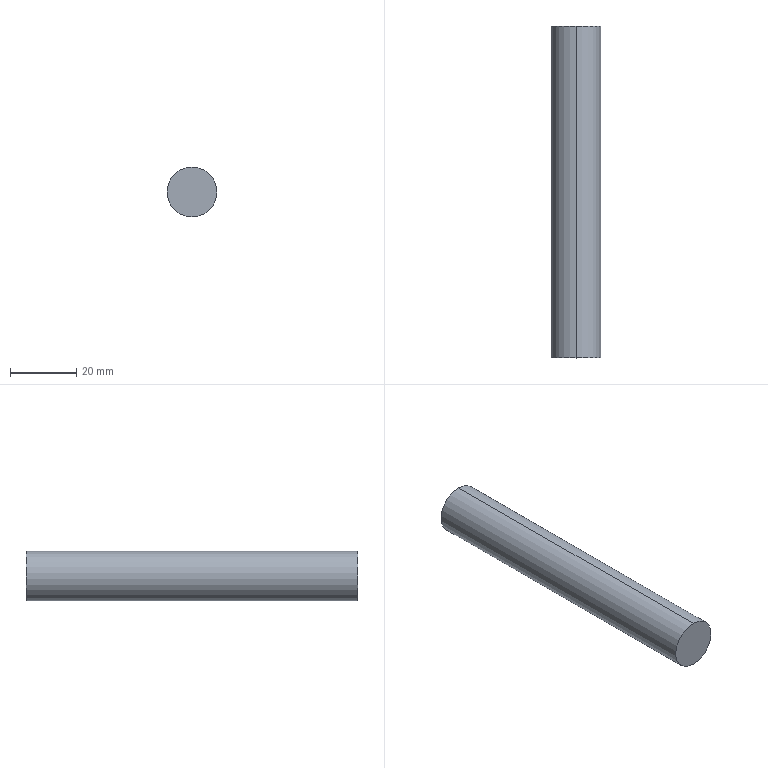Part | SolidWorks | features BaseBody 1 | 1 solid | 8 faces | box 15 x 100 x 15 mm | volume 16839 mm3 | cylinder 4 | cone 2 | plane 2 | commonest cylinder face diameters 6.8 x2 15 x2
STEP:
#1=CARTESIAN_POINT('',(0.,100.,-7.5));
#2=VERTEX_POINT('',#1);
#3=CARTESIAN_POINT('',(0.,100.,7.5));
#4=VERTEX_POINT('',#3);
#5=CARTESIAN_POINT('',(0.,100.,0.));
#6=DIRECTION('',(0.,-1.,0.));
#7=DIRECTION('',(0.,0.,-1.));
#8=AXIS2_PLACEMENT_3D('',#5,#6,#7);
#9=CIRCLE('',#8,7.5);
#10=EDGE_CURVE('',#2,#4,#9,.T.);
#11=ORIENTED_EDGE('',*,*,#10,.T.);
#12=CARTESIAN_POINT('',(0.,0.,7.5));
#13=VERTEX_POINT('',#12);
#14=CARTESIAN_POINT('',(0.,100.,7.5));
#15=DIRECTION('',(0.,-1.,0.));
#16=VECTOR('',#15,1000.);
#17=LINE('',#14,#16);
#18=EDGE_CURVE('',#4,#13,#17,.T.);
#19=ORIENTED_EDGE('',*,*,#18,.T.);
#20=CARTESIAN_POINT('',(0.,0.,-7.5));
#21=VERTEX_POINT('',#20);
#22=CARTESIAN_POINT('',(0.,0.,0.));
#23=DIRECTION('',(0.,1.,0.));
#24=DIRECTION('',(0.,0.,-1.));
#25=AXIS2_PLACEMENT_3D('',#22,#23,#24);
#26=CIRCLE('',#25,7.5);
#27=EDGE_CURVE('',#13,#21,#26,.T.);
#28=ORIENTED_EDGE('',*,*,#27,.T.);
#29=CARTESIAN_POINT('',(0.,100.,-7.5));
#30=DIRECTION('',(0.,-1.,0.));
#31=VECTOR('',#30,1000.);
#32=LINE('',#29,#31);
#33=EDGE_CURVE('',#2,#21,#32,.T.);
#34=ORIENTED_EDGE('',*,*,#33,.F.);
#35=EDGE_LOOP('',(#11,#19,#28,#34));
#36=FACE_OUTER_BOUND('',#35,.T.);
#37=CARTESIAN_POINT('',(0.,100.,0.));
#38=DIRECTION('',(0.,-1.,0.));
#39=DIRECTION('',(0.,0.,-1.));
#40=AXIS2_PLACEMENT_3D('',#37,#38,#39);
#41=CYLINDRICAL_SURFACE('',#40,7.5);
#42=ADVANCED_FACE('',(#36),#41,.T.);
#43=CARTESIAN_POINT('',(0.,77.75,-3.4));
#44=VERTEX_POINT('',#43);
#45=CARTESIAN_POINT('',(0.,77.75,3.4));
#46=VERTEX_POINT('',#45);
#47=CARTESIAN_POINT('',(0.,77.75,0.));
#48=DIRECTION('',(0.,1.,0.));
#49=DIRECTION('',(0.,0.,1.));
#50=AXIS2_PLACEMENT_3D('',#47,#48,#49);
#51=CIRCLE('',#50,3.4);
#52=EDGE_CURVE('',#44,#46,#51,.T.);
#53=ORIENTED_EDGE('',*,*,#52,.F.);
#54=CARTESIAN_POINT('',(0.,100.,-3.4));
#55=VERTEX_POINT('',#54);
#56=CARTESIAN_POINT('',(0.,100.,-3.4));
#57=DIRECTION('',(0.,1.,0.));
#58=VECTOR('',#57,1000.);
#59=LINE('',#56,#58);
#60=EDGE_CURVE('',#44,#55,#59,.T.);
#61=ORIENTED_EDGE('',*,*,#60,.T.);
#62=CARTESIAN_POINT('',(0.,100.,3.4));
#63=VERTEX_POINT('',#62);
#64=CARTESIAN_POINT('',(0.,100.,0.));
#65=DIRECTION('',(0.,-1.,0.));
#66=DIRECTION('',(0.,0.,1.));
#67=AXIS2_PLACEMENT_3D('',#64,#65,#66);
#68=CIRCLE('',#67,3.4);
#69=EDGE_CURVE('',#63,#55,#68,.T.);
#70=ORIENTED_EDGE('',*,*,#69,.F.);
#71=CARTESIAN_POINT('',(0.,100.,3.4));
#72=DIRECTION('',(0.,1.,0.));
#73=VECTOR('',#72,1000.);
#74=LINE('',#71,#73);
#75=EDGE_CURVE('',#46,#63,#74,.T.);
#76=ORIENTED_EDGE('',*,*,#75,.F.);
#77=EDGE_LOOP('',(#53,#61,#70,#76));
#78=FACE_OUTER_BOUND('',#77,.T.);
#79=CARTESIAN_POINT('',(0.,100.,0.));
#80=DIRECTION('',(0.,1.,0.));
#81=DIRECTION('',(0.,0.,1.));
#82=AXIS2_PLACEMENT_3D('',#79,#80,#81);
#83=CYLINDRICAL_SURFACE('',#82,3.4);
#84=ADVANCED_FACE('',(#78),#83,.F.);
#85=CARTESIAN_POINT('',(0.,75.707,0.));
#86=VERTEX_POINT('',#85);
#87=CARTESIAN_POINT('',(0.,77.75,3.4));
#88=DIRECTION('',(0.,0.515,0.8572));
#89=VECTOR('',#88,1000.);
#90=LINE('',#87,#89);
#91=EDGE_CURVE('',#86,#46,#90,.T.);
#92=ORIENTED_EDGE('',*,*,#91,.F.);
#93=CARTESIAN_POINT('',(0.,77.75,-3.4));
#94=DIRECTION('',(0.,0.515,-0.8572));
#95=VECTOR('',#94,1000.);
#96=LINE('',#93,#95);
#97=EDGE_CURVE('',#86,#44,#96,.T.);
#98=ORIENTED_EDGE('',*,*,#97,.T.);
#99=ORIENTED_EDGE('',*,*,#52,.T.);
#100=EDGE_LOOP('',(#92,#98,#99));
#101=FACE_OUTER_BOUND('',#100,.T.);
#102=CARTESIAN_POINT('',(0.,77.75,0.));
#103=DIRECTION('',(0.,1.,0.));
#104=DIRECTION('',(0.,0.,1.));
#105=AXIS2_PLACEMENT_3D('',#102,#103,#104);
#106=CONICAL_SURFACE('',#105,3.4,1.03);
#107=ADVANCED_FACE('',(#101),#106,.F.);
#108=ORIENTED_EDGE('',*,*,#18,.F.);
#109=CARTESIAN_POINT('',(0.,100.,0.));
#110=DIRECTION('',(0.,-1.,0.));
#111=DIRECTION('',(0.,0.,-1.));
#112=AXIS2_PLACEMENT_3D('',#109,#110,#111);
#113=CIRCLE('',#112,7.5);
#114=EDGE_CURVE('',#4,#2,#113,.T.);
#115=ORIENTED_EDGE('',*,*,#114,.T.);
#116=ORIENTED_EDGE('',*,*,#33,.T.);
#117=CARTESIAN_POINT('',(0.,0.,0.));
#118=DIRECTION('',(0.,1.,0.));
#119=DIRECTION('',(0.,0.,-1.));
#120=AXIS2_PLACEMENT_3D('',#117,#118,#119);
#121=CIRCLE('',#120,7.5);
#122=EDGE_CURVE('',#21,#13,#121,.T.);
#123=ORIENTED_EDGE('',*,*,#122,.T.);
#124=EDGE_LOOP('',(#108,#115,#116,#123));
#125=FACE_OUTER_BOUND('',#124,.T.);
#126=CARTESIAN_POINT('',(0.,100.,0.));
#127=DIRECTION('',(0.,-1.,0.));
#128=DIRECTION('',(0.,0.,-1.));
#129=AXIS2_PLACEMENT_3D('',#126,#127,#128);
#130=CYLINDRICAL_SURFACE('',#129,7.5);
#131=ADVANCED_FACE('',(#125),#130,.T.);
#132=ORIENTED_EDGE('',*,*,#122,.F.);
#133=ORIENTED_EDGE('',*,*,#27,.F.);
#134=EDGE_LOOP('',(#132,#133));
#135=FACE_OUTER_BOUND('',#134,.T.);
#136=CARTESIAN_POINT('',(0.,0.,0.));
#137=DIRECTION('',(0.,1.,0.));
#138=DIRECTION('',(0.,0.,1.));
#139=AXIS2_PLACEMENT_3D('',#136,#137,#138);
#140=PLANE('',#139);
#141=ADVANCED_FACE('',(#135),#140,.F.);
#142=ORIENTED_EDGE('',*,*,#10,.F.);
#143=ORIENTED_EDGE('',*,*,#114,.F.);
#144=EDGE_LOOP('',(#142,#143));
#145=FACE_OUTER_BOUND('',#144,.T.);
#146=ORIENTED_EDGE('',*,*,#69,.T.);
#147=CARTESIAN_POINT('',(0.,100.,0.));
#148=DIRECTION('',(0.,-1.,0.));
#149=DIRECTION('',(0.,0.,1.));
#150=AXIS2_PLACEMENT_3D('',#147,#148,#149);
#151=CIRCLE('',#150,3.4);
#152=EDGE_CURVE('',#55,#63,#151,.T.);
#153=ORIENTED_EDGE('',*,*,#152,.T.);
#154=EDGE_LOOP('',(#146,#153));
#155=FACE_BOUND('',#154,.T.);
#156=CARTESIAN_POINT('',(0.,100.,0.));
#157=DIRECTION('',(0.,1.,0.));
#158=DIRECTION('',(0.,0.,1.));
#159=AXIS2_PLACEMENT_3D('',#156,#157,#158);
#160=PLANE('',#159);
#161=ADVANCED_FACE('',(#145,#155),#160,.T.);
#162=ORIENTED_EDGE('',*,*,#60,.F.);
#163=CARTESIAN_POINT('',(0.,77.75,0.));
#164=DIRECTION('',(0.,1.,0.));
#165=DIRECTION('',(0.,0.,1.));
#166=AXIS2_PLACEMENT_3D('',#163,#164,#165);
#167=CIRCLE('',#166,3.4);
#168=EDGE_CURVE('',#46,#44,#167,.T.);
#169=ORIENTED_EDGE('',*,*,#168,.F.);
#170=ORIENTED_EDGE('',*,*,#75,.T.);
#171=ORIENTED_EDGE('',*,*,#152,.F.);
#172=EDGE_LOOP('',(#162,#169,#170,#171));
#173=FACE_OUTER_BOUND('',#172,.T.);
#174=CARTESIAN_POINT('',(0.,100.,0.));
#175=DIRECTION('',(0.,1.,0.));
#176=DIRECTION('',(0.,0.,1.));
#177=AXIS2_PLACEMENT_3D('',#174,#175,#176);
#178=CYLINDRICAL_SURFACE('',#177,3.4);
#179=ADVANCED_FACE('',(#173),#178,.F.);
#180=ORIENTED_EDGE('',*,*,#97,.F.);
#181=ORIENTED_EDGE('',*,*,#91,.T.);
#182=ORIENTED_EDGE('',*,*,#168,.T.);
#183=EDGE_LOOP('',(#180,#181,#182));
#184=FACE_OUTER_BOUND('',#183,.T.);
#185=CARTESIAN_POINT('',(0.,77.75,0.));
#186=DIRECTION('',(0.,1.,0.));
#187=DIRECTION('',(0.,0.,1.));
#188=AXIS2_PLACEMENT_3D('',#185,#186,#187);
#189=CONICAL_SURFACE('',#188,3.4,1.03);
#190=ADVANCED_FACE('',(#184),#189,.F.);
#191=CLOSED_SHELL('',(#42,#84,#107,#131,#141,#161,#179,#190));
#192=MANIFOLD_SOLID_BREP('',#191);
#193=CARTESIAN_POINT('',(0.,0.,0.));
#194=DIRECTION('',(0.,0.,1.));
#195=DIRECTION('',(1.,0.,0.));
#196=AXIS2_PLACEMENT_3D('',#193,#194,#195);
#197=(LENGTH_UNIT()NAMED_UNIT(*)SI_UNIT(.MILLI.,.METRE.));
#198=UNCERTAINTY_MEASURE_WITH_UNIT(LENGTH_MEASURE(0.00001),#197,'','');
#199=(NAMED_UNIT(*)PLANE_ANGLE_UNIT()SI_UNIT($,.RADIAN.));
#200=(NAMED_UNIT(*)SI_UNIT($,.STERADIAN.)SOLID_ANGLE_UNIT());
#201=(GEOMETRIC_REPRESENTATION_CONTEXT(3)GLOBAL_UNCERTAINTY_ASSIGNED_CONTEXT((#198))GLOBAL_UNIT_ASSIGNED_CONTEXT((#197,#199,#200))REPRESENTATION_CONTEXT('',''));
#202=ADVANCED_BREP_SHAPE_REPRESENTATION('',(#192,#196),#201);